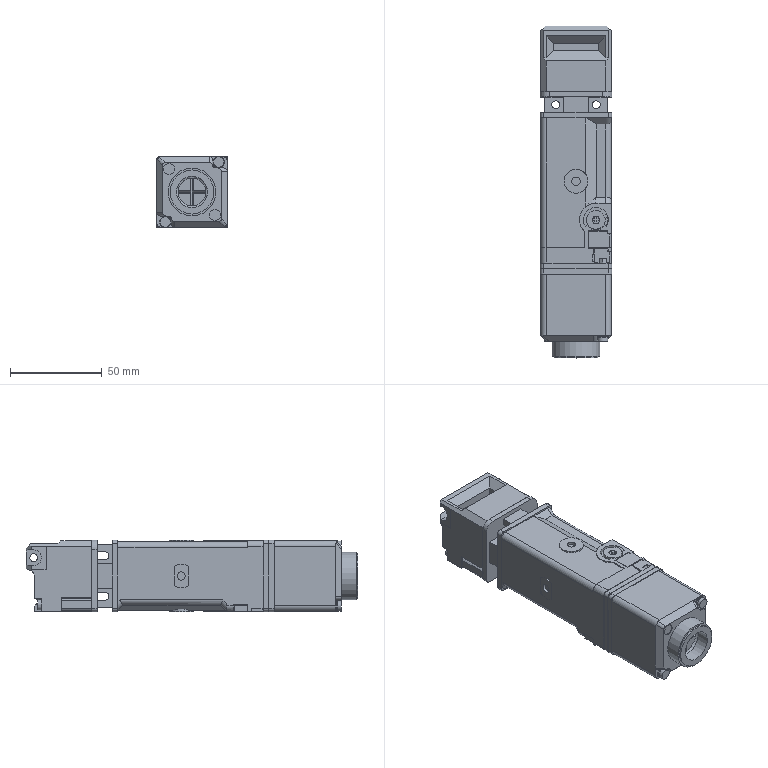Part | NX | 1 solid | 501 faces | box 39 x 180.9 x 39.045 mm | volume 229791 mm3 | plane 397 | cylinder 100 | spline 2 | cone 1 | torus 1 | commonest cylinder face diameters 4 x22 6 x19 13 x8 7.4 x6 7.6 x6 4.3 x5